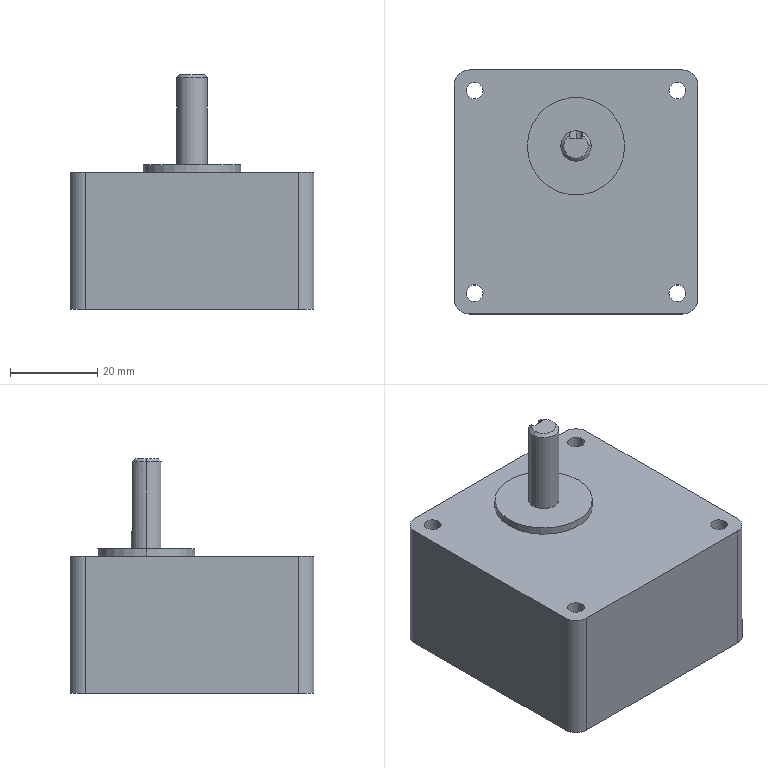Part | SolidWorks | features SplitBody 1 | 1 solid | 32 faces | box 56 x 56 x 53.9 mm | volume 98386 mm3 | cylinder 18 | plane 11 | cone 3 | commonest cylinder face diameters 3.85 x8 7 x6 2.8 x2 22.4 x2
STEP:
#1=CARTESIAN_POINT('',(-31.203,204.359,-234.916));
#2=VERTEX_POINT('',#1);
#3=CARTESIAN_POINT('',(-32.603,206.784,-234.916));
#4=VERTEX_POINT('',#3);
#5=CARTESIAN_POINT('',(-34.003,204.359,-234.916));
#6=DIRECTION('',(0.,0.,1.));
#7=DIRECTION('',(1.,0.,0.));
#8=AXIS2_PLACEMENT_3D('',#5,#6,#7);
#9=CIRCLE('',#8,2.8);
#10=EDGE_CURVE('',#2,#4,#9,.T.);
#11=ORIENTED_EDGE('',*,*,#10,.F.);
#12=CARTESIAN_POINT('',(-30.503,204.359,-235.616));
#13=VERTEX_POINT('',#12);
#14=CARTESIAN_POINT('',(-31.203,204.359,-234.916));
#15=DIRECTION('',(0.7071,0.,-0.7071));
#16=VECTOR('',#15,1000.);
#17=LINE('',#14,#16);
#18=EDGE_CURVE('',#2,#13,#17,.T.);
#19=ORIENTED_EDGE('',*,*,#18,.T.);
#20=CARTESIAN_POINT('',(-32.603,207.567,-235.616));
#21=VERTEX_POINT('',#20);
#22=CARTESIAN_POINT('',(-34.003,204.359,-235.616));
#23=DIRECTION('',(0.,0.,-1.));
#24=DIRECTION('',(1.,0.,0.));
#25=AXIS2_PLACEMENT_3D('',#22,#23,#24);
#26=CIRCLE('',#25,3.5);
#27=EDGE_CURVE('',#21,#13,#26,.T.);
#28=ORIENTED_EDGE('',*,*,#27,.F.);
#29=CARTESIAN_POINT('',(-32.603,206.784,-234.916));
#30=CARTESIAN_POINT('',(-32.603,207.049,-235.145));
#31=CARTESIAN_POINT('',(-32.603,207.309,-235.379));
#32=CARTESIAN_POINT('',(-32.603,207.567,-235.616));
#33=B_SPLINE_CURVE_WITH_KNOTS('',3,(#29,#30,#31,#32),.UNSPECIFIED.,.F.,.F.,(4,4),(0.002327,0.00337),.UNSPECIFIED.);
#34=EDGE_CURVE('',#4,#21,#33,.T.);
#35=ORIENTED_EDGE('',*,*,#34,.F.);
#36=EDGE_LOOP('',(#11,#19,#28,#35));
#37=FACE_OUTER_BOUND('',#36,.T.);
#38=CARTESIAN_POINT('',(-34.003,204.359,-234.916));
#39=DIRECTION('',(0.,0.,-1.));
#40=DIRECTION('',(-1.,0.,0.));
#41=AXIS2_PLACEMENT_3D('',#38,#39,#40);
#42=CONICAL_SURFACE('',#41,2.8,0.7854);
#43=ADVANCED_FACE('',(#37),#42,.T.);
#44=ORIENTED_EDGE('',*,*,#18,.F.);
#45=CARTESIAN_POINT('',(-36.803,204.359,-234.916));
#46=VERTEX_POINT('',#45);
#47=CARTESIAN_POINT('',(-34.003,204.359,-234.916));
#48=DIRECTION('',(0.,0.,1.));
#49=DIRECTION('',(1.,0.,0.));
#50=AXIS2_PLACEMENT_3D('',#47,#48,#49);
#51=CIRCLE('',#50,2.8);
#52=EDGE_CURVE('',#46,#2,#51,.T.);
#53=ORIENTED_EDGE('',*,*,#52,.F.);
#54=CARTESIAN_POINT('',(-37.503,204.359,-235.616));
#55=VERTEX_POINT('',#54);
#56=CARTESIAN_POINT('',(-36.803,204.359,-234.916));
#57=DIRECTION('',(-0.7071,0.,-0.7071));
#58=VECTOR('',#57,1000.);
#59=LINE('',#56,#58);
#60=EDGE_CURVE('',#46,#55,#59,.T.);
#61=ORIENTED_EDGE('',*,*,#60,.T.);
#62=CARTESIAN_POINT('',(-34.003,204.359,-235.616));
#63=DIRECTION('',(0.,0.,-1.));
#64=DIRECTION('',(1.,0.,0.));
#65=AXIS2_PLACEMENT_3D('',#62,#63,#64);
#66=CIRCLE('',#65,3.5);
#67=EDGE_CURVE('',#13,#55,#66,.T.);
#68=ORIENTED_EDGE('',*,*,#67,.F.);
#69=EDGE_LOOP('',(#44,#53,#61,#68));
#70=FACE_OUTER_BOUND('',#69,.T.);
#71=CARTESIAN_POINT('',(-34.003,204.359,-234.916));
#72=DIRECTION('',(0.,0.,-1.));
#73=DIRECTION('',(-1.,0.,0.));
#74=AXIS2_PLACEMENT_3D('',#71,#72,#73);
#75=CONICAL_SURFACE('',#74,2.8,0.7854);
#76=ADVANCED_FACE('',(#70),#75,.T.);
#77=ORIENTED_EDGE('',*,*,#27,.T.);
#78=CARTESIAN_POINT('',(-30.503,204.359,-255.566));
#79=VERTEX_POINT('',#78);
#80=CARTESIAN_POINT('',(-30.503,204.359,-234.916));
#81=DIRECTION('',(0.,0.,-1.));
#82=VECTOR('',#81,1000.);
#83=LINE('',#80,#82);
#84=EDGE_CURVE('',#13,#79,#83,.T.);
#85=ORIENTED_EDGE('',*,*,#84,.T.);
#86=CARTESIAN_POINT('',(-37.503,204.359,-255.566));
#87=VERTEX_POINT('',#86);
#88=CARTESIAN_POINT('',(-34.003,204.359,-255.566));
#89=DIRECTION('',(0.,0.,-1.));
#90=DIRECTION('',(1.,0.,0.));
#91=AXIS2_PLACEMENT_3D('',#88,#89,#90);
#92=CIRCLE('',#91,3.5);
#93=EDGE_CURVE('',#87,#79,#92,.T.);
#94=ORIENTED_EDGE('',*,*,#93,.F.);
#95=CARTESIAN_POINT('',(-37.503,204.359,-234.916));
#96=DIRECTION('',(0.,0.,-1.));
#97=VECTOR('',#96,1000.);
#98=LINE('',#95,#97);
#99=EDGE_CURVE('',#55,#87,#98,.T.);
#100=ORIENTED_EDGE('',*,*,#99,.F.);
#101=CARTESIAN_POINT('',(-35.403,207.567,-235.616));
#102=VERTEX_POINT('',#101);
#103=CARTESIAN_POINT('',(-34.003,204.359,-235.616));
#104=DIRECTION('',(0.,0.,-1.));
#105=DIRECTION('',(1.,0.,0.));
#106=AXIS2_PLACEMENT_3D('',#103,#104,#105);
#107=CIRCLE('',#106,3.5);
#108=EDGE_CURVE('',#55,#102,#107,.T.);
#109=ORIENTED_EDGE('',*,*,#108,.T.);
#110=CARTESIAN_POINT('',(-35.403,207.567,-251.016));
#111=VERTEX_POINT('',#110);
#112=CARTESIAN_POINT('',(-35.403,207.567,-234.916));
#113=DIRECTION('',(0.,0.,-1.));
#114=VECTOR('',#113,1000.);
#115=LINE('',#112,#114);
#116=EDGE_CURVE('',#102,#111,#115,.T.);
#117=ORIENTED_EDGE('',*,*,#116,.T.);
#118=CARTESIAN_POINT('',(-34.003,207.859,-252.416));
#119=VERTEX_POINT('',#118);
#120=CARTESIAN_POINT('',(-35.403,207.567,-251.016));
#121=CARTESIAN_POINT('',(-35.403,207.567,-251.109));
#122=CARTESIAN_POINT('',(-35.394,207.571,-251.201));
#123=CARTESIAN_POINT('',(-35.357,207.586,-251.381));
#124=CARTESIAN_POINT('',(-35.33,207.598,-251.47));
#125=CARTESIAN_POINT('',(-35.224,207.64,-251.724));
#126=CARTESIAN_POINT('',(-35.121,207.678,-251.877));
#127=CARTESIAN_POINT('',(-34.866,207.754,-252.133));
#128=CARTESIAN_POINT('',(-34.711,207.791,-252.237));
#129=CARTESIAN_POINT('',(-34.375,207.843,-252.377));
#130=CARTESIAN_POINT('',(-34.19,207.859,-252.416));
#131=CARTESIAN_POINT('',(-34.003,207.859,-252.416));
#132=B_SPLINE_CURVE_WITH_KNOTS('',3,(#120,#121,#122,#123,#124,#125,#126,#127,#128,#129,#130,#131),.UNSPECIFIED.,.F.,.F.,(4,2,2,2,2,4),(0.,0.0002763,0.0005526,0.001105,0.001658,0.00221),.UNSPECIFIED.);
#133=EDGE_CURVE('',#111,#119,#132,.T.);
#134=ORIENTED_EDGE('',*,*,#133,.T.);
#135=CARTESIAN_POINT('',(-32.603,207.567,-251.016));
#136=VERTEX_POINT('',#135);
#137=CARTESIAN_POINT('',(-34.003,207.859,-252.416));
#138=CARTESIAN_POINT('',(-33.909,207.859,-252.416));
#139=CARTESIAN_POINT('',(-33.818,207.855,-252.406));
#140=CARTESIAN_POINT('',(-33.637,207.841,-252.37));
#141=CARTESIAN_POINT('',(-33.548,207.83,-252.343));
#142=CARTESIAN_POINT('',(-33.294,207.791,-252.237));
#143=CARTESIAN_POINT('',(-33.14,207.754,-252.133));
#144=CARTESIAN_POINT('',(-32.885,207.678,-251.878));
#145=CARTESIAN_POINT('',(-32.781,207.64,-251.723));
#146=CARTESIAN_POINT('',(-32.641,207.584,-251.388));
#147=CARTESIAN_POINT('',(-32.603,207.567,-251.203));
#148=CARTESIAN_POINT('',(-32.603,207.567,-251.016));
#149=B_SPLINE_CURVE_WITH_KNOTS('',3,(#137,#138,#139,#140,#141,#142,#143,#144,#145,#146,#147,#148),.UNSPECIFIED.,.F.,.F.,(4,2,2,2,2,4),(0.,0.0002763,0.0005527,0.001105,0.001658,0.002211),.UNSPECIFIED.);
#150=EDGE_CURVE('',#119,#136,#149,.T.);
#151=ORIENTED_EDGE('',*,*,#150,.T.);
#152=CARTESIAN_POINT('',(-32.603,207.567,-234.916));
#153=DIRECTION('',(0.,0.,1.));
#154=VECTOR('',#153,1000.);
#155=LINE('',#152,#154);
#156=EDGE_CURVE('',#136,#21,#155,.T.);
#157=ORIENTED_EDGE('',*,*,#156,.T.);
#158=EDGE_LOOP('',(#77,#85,#94,#100,#109,#117,#134,#151,#157));
#159=FACE_OUTER_BOUND('',#158,.T.);
#160=CARTESIAN_POINT('',(-34.003,204.359,-234.916));
#161=DIRECTION('',(0.,0.,-1.));
#162=DIRECTION('',(-1.,0.,0.));
#163=AXIS2_PLACEMENT_3D('',#160,#161,#162);
#164=CYLINDRICAL_SURFACE('',#163,3.5);
#165=ADVANCED_FACE('',(#159),#164,.T.);
#166=CARTESIAN_POINT('',(-22.803,204.359,-255.566));
#167=VERTEX_POINT('',#166);
#168=CARTESIAN_POINT('',(-45.203,204.359,-255.566));
#169=VERTEX_POINT('',#168);
#170=CARTESIAN_POINT('',(-34.003,204.359,-255.566));
#171=DIRECTION('',(0.,0.,1.));
#172=DIRECTION('',(1.,0.,0.));
#173=AXIS2_PLACEMENT_3D('',#170,#171,#172);
#174=CIRCLE('',#173,11.2);
#175=EDGE_CURVE('',#167,#169,#174,.T.);
#176=ORIENTED_EDGE('',*,*,#175,.F.);
#177=CARTESIAN_POINT('',(-22.803,204.359,-257.316));
#178=VERTEX_POINT('',#177);
#179=CARTESIAN_POINT('',(-22.803,204.359,-255.566));
#180=DIRECTION('',(0.,0.,-1.));
#181=VECTOR('',#180,1000.);
#182=LINE('',#179,#181);
#183=EDGE_CURVE('',#167,#178,#182,.T.);
#184=ORIENTED_EDGE('',*,*,#183,.T.);
#185=CARTESIAN_POINT('',(-45.203,204.359,-257.316));
#186=VERTEX_POINT('',#185);
#187=CARTESIAN_POINT('',(-34.003,204.359,-257.316));
#188=DIRECTION('',(0.,0.,1.));
#189=DIRECTION('',(1.,0.,0.));
#190=AXIS2_PLACEMENT_3D('',#187,#188,#189);
#191=CIRCLE('',#190,11.2);
#192=EDGE_CURVE('',#178,#186,#191,.T.);
#193=ORIENTED_EDGE('',*,*,#192,.T.);
#194=CARTESIAN_POINT('',(-45.203,204.359,-255.566));
#195=DIRECTION('',(0.,0.,-1.));
#196=VECTOR('',#195,1000.);
#197=LINE('',#194,#196);
#198=EDGE_CURVE('',#169,#186,#197,.T.);
#199=ORIENTED_EDGE('',*,*,#198,.F.);
#200=EDGE_LOOP('',(#176,#184,#193,#199));
#201=FACE_OUTER_BOUND('',#200,.T.);
#202=CARTESIAN_POINT('',(-34.003,204.359,-255.566));
#203=DIRECTION('',(0.,0.,-1.));
#204=DIRECTION('',(-1.,0.,0.));
#205=AXIS2_PLACEMENT_3D('',#202,#203,#204);
#206=CYLINDRICAL_SURFACE('',#205,11.2);
#207=ADVANCED_FACE('',(#201),#206,.T.);
#208=CARTESIAN_POINT('',(-12.664,217.123,-257.316));
#209=VERTEX_POINT('',#208);
#210=CARTESIAN_POINT('',(-8.814,217.123,-257.316));
#211=VERTEX_POINT('',#210);
#212=CARTESIAN_POINT('',(-10.739,217.123,-257.316));
#213=DIRECTION('',(0.,0.,1.));
#214=DIRECTION('',(1.,0.,0.));
#215=AXIS2_PLACEMENT_3D('',#212,#213,#214);
#216=CIRCLE('',#215,1.925);
#217=EDGE_CURVE('',#209,#211,#216,.T.);
#218=ORIENTED_EDGE('',*,*,#217,.T.);
#219=CARTESIAN_POINT('',(-8.814,217.123,-288.816));
#220=VERTEX_POINT('',#219);
#221=CARTESIAN_POINT('',(-8.814,217.123,-257.316));
#222=DIRECTION('',(0.,0.,-1.));
#223=VECTOR('',#222,1000.);
#224=LINE('',#221,#223);
#225=EDGE_CURVE('',#211,#220,#224,.T.);
#226=ORIENTED_EDGE('',*,*,#225,.T.);
#227=CARTESIAN_POINT('',(-12.664,217.123,-288.816));
#228=VERTEX_POINT('',#227);
#229=CARTESIAN_POINT('',(-10.739,217.123,-288.816));
#230=DIRECTION('',(0.,0.,1.));
#231=DIRECTION('',(1.,0.,0.));
#232=AXIS2_PLACEMENT_3D('',#229,#230,#231);
#233=CIRCLE('',#232,1.925);
#234=EDGE_CURVE('',#228,#220,#233,.T.);
#235=ORIENTED_EDGE('',*,*,#234,.F.);
#236=CARTESIAN_POINT('',(-12.664,217.123,-257.316));
#237=DIRECTION('',(0.,0.,-1.));
#238=VECTOR('',#237,1000.);
#239=LINE('',#236,#238);
#240=EDGE_CURVE('',#209,#228,#239,.T.);
#241=ORIENTED_EDGE('',*,*,#240,.F.);
#242=EDGE_LOOP('',(#218,#226,#235,#241));
#243=FACE_OUTER_BOUND('',#242,.T.);
#244=CARTESIAN_POINT('',(-10.739,217.123,-257.316));
#245=DIRECTION('',(0.,0.,-1.));
#246=DIRECTION('',(-1.,0.,0.));
#247=AXIS2_PLACEMENT_3D('',#244,#245,#246);
#248=CYLINDRICAL_SURFACE('',#247,1.925);
#249=ADVANCED_FACE('',(#243),#248,.F.);
#250=CARTESIAN_POINT('',(-12.664,170.595,-257.316));
#251=VERTEX_POINT('',#250);
#252=CARTESIAN_POINT('',(-8.814,170.595,-257.316));
#253=VERTEX_POINT('',#252);
#254=CARTESIAN_POINT('',(-10.739,170.595,-257.316));
#255=DIRECTION('',(0.,0.,1.));
#256=DIRECTION('',(1.,0.,0.));
#257=AXIS2_PLACEMENT_3D('',#254,#255,#256);
#258=CIRCLE('',#257,1.925);
#259=EDGE_CURVE('',#251,#253,#258,.T.);
#260=ORIENTED_EDGE('',*,*,#259,.T.);
#261=CARTESIAN_POINT('',(-8.814,170.595,-288.816));
#262=VERTEX_POINT('',#261);
#263=CARTESIAN_POINT('',(-8.814,170.595,-257.316));
#264=DIRECTION('',(0.,0.,-1.));
#265=VECTOR('',#264,1000.);
#266=LINE('',#263,#265);
#267=EDGE_CURVE('',#253,#262,#266,.T.);
#268=ORIENTED_EDGE('',*,*,#267,.T.);
#269=CARTESIAN_POINT('',(-12.664,170.595,-288.816));
#270=VERTEX_POINT('',#269);
#271=CARTESIAN_POINT('',(-10.739,170.595,-288.816));
#272=DIRECTION('',(0.,0.,1.));
#273=DIRECTION('',(1.,0.,0.));
#274=AXIS2_PLACEMENT_3D('',#271,#272,#273);
#275=CIRCLE('',#274,1.925);
#276=EDGE_CURVE('',#270,#262,#275,.T.);
#277=ORIENTED_EDGE('',*,*,#276,.F.);
#278=CARTESIAN_POINT('',(-12.664,170.595,-257.316));
#279=DIRECTION('',(0.,0.,-1.));
#280=VECTOR('',#279,1000.);
#281=LINE('',#278,#280);
#282=EDGE_CURVE('',#251,#270,#281,.T.);
#283=ORIENTED_EDGE('',*,*,#282,.F.);
#284=EDGE_LOOP('',(#260,#268,#277,#283));
#285=FACE_OUTER_BOUND('',#284,.T.);
#286=CARTESIAN_POINT('',(-10.739,170.595,-257.316));
#287=DIRECTION('',(0.,0.,-1.));
#288=DIRECTION('',(-1.,0.,0.));
#289=AXIS2_PLACEMENT_3D('',#286,#287,#288);
#290=CYLINDRICAL_SURFACE('',#289,1.925);
#291=ADVANCED_FACE('',(#285),#290,.F.);
#292=CARTESIAN_POINT('',(-59.192,170.595,-257.316));
#293=VERTEX_POINT('',#292);
#294=CARTESIAN_POINT('',(-55.342,170.595,-257.316));
#295=VERTEX_POINT('',#294);
#296=CARTESIAN_POINT('',(-57.267,170.595,-257.316));
#297=DIRECTION('',(0.,0.,1.));
#298=DIRECTION('',(1.,0.,0.));
#299=AXIS2_PLACEMENT_3D('',#296,#297,#298);
#300=CIRCLE('',#299,1.925);
#301=EDGE_CURVE('',#293,#295,#300,.T.);
#302=ORIENTED_EDGE('',*,*,#301,.T.);
#303=CARTESIAN_POINT('',(-55.342,170.595,-288.816));
#304=VERTEX_POINT('',#303);
#305=CARTESIAN_POINT('',(-55.342,170.595,-257.316));
#306=DIRECTION('',(0.,0.,-1.));
#307=VECTOR('',#306,1000.);
#308=LINE('',#305,#307);
#309=EDGE_CURVE('',#295,#304,#308,.T.);
#310=ORIENTED_EDGE('',*,*,#309,.T.);
#311=CARTESIAN_POINT('',(-59.192,170.595,-288.816));
#312=VERTEX_POINT('',#311);
#313=CARTESIAN_POINT('',(-57.267,170.595,-288.816));
#314=DIRECTION('',(0.,0.,1.));
#315=DIRECTION('',(1.,0.,0.));
#316=AXIS2_PLACEMENT_3D('',#313,#314,#315);
#317=CIRCLE('',#316,1.925);
#318=EDGE_CURVE('',#312,#304,#317,.T.);
#319=ORIENTED_EDGE('',*,*,#318,.F.);
#320=CARTESIAN_POINT('',(-59.192,170.595,-257.316));
#321=DIRECTION('',(0.,0.,-1.));
#322=VECTOR('',#321,1000.);
#323=LINE('',#320,#322);
#324=EDGE_CURVE('',#293,#312,#323,.T.);
#325=ORIENTED_EDGE('',*,*,#324,.F.);
#326=EDGE_LOOP('',(#302,#310,#319,#325));
#327=FACE_OUTER_BOUND('',#326,.T.);
#328=CARTESIAN_POINT('',(-57.267,170.595,-257.316));
#329=DIRECTION('',(0.,0.,-1.));
#330=DIRECTION('',(-1.,0.,0.));
#331=AXIS2_PLACEMENT_3D('',#328,#329,#330);
#332=CYLINDRICAL_SURFACE('',#331,1.925);
#333=ADVANCED_FACE('',(#327),#332,.F.);
#334=CARTESIAN_POINT('',(-59.192,217.123,-257.316));
#335=VERTEX_POINT('',#334);
#336=CARTESIAN_POINT('',(-55.342,217.123,-257.316));
#337=VERTEX_POINT('',#336);
#338=CARTESIAN_POINT('',(-57.267,217.123,-257.316));
#339=DIRECTION('',(0.,0.,1.));
#340=DIRECTION('',(1.,0.,0.));
#341=AXIS2_PLACEMENT_3D('',#338,#339,#340);
#342=CIRCLE('',#341,1.925);
#343=EDGE_CURVE('',#335,#337,#342,.T.);
#344=ORIENTED_EDGE('',*,*,#343,.T.);
#345=CARTESIAN_POINT('',(-55.342,217.123,-288.816));
#346=VERTEX_POINT('',#345);
#347=CARTESIAN_POINT('',(-55.342,217.123,-257.316));
#348=DIRECTION('',(0.,0.,-1.));
#349=VECTOR('',#348,1000.);
#350=LINE('',#347,#349);
#351=EDGE_CURVE('',#337,#346,#350,.T.);
#352=ORIENTED_EDGE('',*,*,#351,.T.);
#353=CARTESIAN_POINT('',(-59.192,217.123,-288.816));
#354=VERTEX_POINT('',#353);
#355=CARTESIAN_POINT('',(-57.267,217.123,-288.816));
#356=DIRECTION('',(0.,0.,1.));
#357=DIRECTION('',(1.,0.,0.));
#358=AXIS2_PLACEMENT_3D('',#355,#356,#357);
#359=CIRCLE('',#358,1.925);
#360=EDGE_CURVE('',#354,#346,#359,.T.);
#361=ORIENTED_EDGE('',*,*,#360,.F.);
#362=CARTESIAN_POINT('',(-59.192,217.123,-257.316));
#363=DIRECTION('',(0.,0.,-1.));
#364=VECTOR('',#363,1000.);
#365=LINE('',#362,#364);
#366=EDGE_CURVE('',#335,#354,#365,.T.);
#367=ORIENTED_EDGE('',*,*,#366,.F.);
#368=EDGE_LOOP('',(#344,#352,#361,#367));
#369=FACE_OUTER_BOUND('',#368,.T.);
#370=CARTESIAN_POINT('',(-57.267,217.123,-257.316));
#371=DIRECTION('',(0.,0.,-1.));
#372=DIRECTION('',(-1.,0.,0.));
#373=AXIS2_PLACEMENT_3D('',#370,#371,#372);
#374=CYLINDRICAL_SURFACE('',#373,1.925);
#375=ADVANCED_FACE('',(#369),#374,.F.);
#376=CARTESIAN_POINT('',(-34.003,204.359,-255.566));
#377=DIRECTION('',(0.,0.,1.));
#378=DIRECTION('',(1.,0.,0.));
#379=AXIS2_PLACEMENT_3D('',#376,#377,#378);
#380=CIRCLE('',#379,11.2);
#381=EDGE_CURVE('',#169,#167,#380,.T.);
#382=ORIENTED_EDGE('',*,*,#381,.T.);
#383=ORIENTED_EDGE('',*,*,#175,.T.);
#384=EDGE_LOOP('',(#382,#383));
#385=FACE_OUTER_BOUND('',#384,.T.);
#386=ORIENTED_EDGE('',*,*,#93,.T.);
#387=CARTESIAN_POINT('',(-34.003,204.359,-255.566));
#388=DIRECTION('',(0.,0.,-1.));
#389=DIRECTION('',(1.,0.,0.));
#390=AXIS2_PLACEMENT_3D('',#387,#388,#389);
#391=CIRCLE('',#390,3.5);
#392=EDGE_CURVE('',#79,#87,#391,.T.);
#393=ORIENTED_EDGE('',*,*,#392,.T.);
#394=EDGE_LOOP('',(#386,#393));
#395=FACE_BOUND('',#394,.T.);
#396=CARTESIAN_POINT('',(-34.003,204.359,-255.566));
#397=DIRECTION('',(0.,0.,1.));
#398=DIRECTION('',(1.,0.,0.));
#399=AXIS2_PLACEMENT_3D('',#396,#397,#398);
#400=PLANE('',#399);
#401=ADVANCED_FACE('',(#385,#395),#400,.T.);
#402=ORIENTED_EDGE('',*,*,#217,.F.);
#403=CARTESIAN_POINT('',(-10.739,217.123,-257.316));
#404=DIRECTION('',(0.,0.,1.));
#405=DIRECTION('',(1.,0.,0.));
#406=AXIS2_PLACEMENT_3D('',#403,#404,#405);
#407=CIRCLE('',#406,1.925);
#408=EDGE_CURVE('',#211,#209,#407,.T.);
#409=ORIENTED_EDGE('',*,*,#408,.F.);
#410=EDGE_LOOP('',(#402,#409));
#411=FACE_BOUND('',#410,.T.);
#412=ORIENTED_EDGE('',*,*,#301,.F.);
#413=CARTESIAN_POINT('',(-57.267,170.595,-257.316));
#414=DIRECTION('',(0.,0.,1.));
#415=DIRECTION('',(1.,0.,0.));
#416=AXIS2_PLACEMENT_3D('',#413,#414,#415);
#417=CIRCLE('',#416,1.925);
#418=EDGE_CURVE('',#295,#293,#417,.T.);
#419=ORIENTED_EDGE('',*,*,#418,.F.);
#420=EDGE_LOOP('',(#412,#419));
#421=FACE_BOUND('',#420,.T.);
#422=CARTESIAN_POINT('',(-62.003,169.359,-257.316));
#423=VERTEX_POINT('',#422);
#424=CARTESIAN_POINT('',(-58.503,165.859,-257.316));
#425=VERTEX_POINT('',#424);
#426=CARTESIAN_POINT('',(-58.503,169.359,-257.316));
#427=DIRECTION('',(0.,0.,1.));
#428=DIRECTION('',(1.,0.,0.));
#429=AXIS2_PLACEMENT_3D('',#426,#427,#428);
#430=CIRCLE('',#429,3.5);
#431=EDGE_CURVE('',#423,#425,#430,.T.);
#432=ORIENTED_EDGE('',*,*,#431,.T.);
#433=CARTESIAN_POINT('',(-9.503,165.859,-257.316));
#434=VERTEX_POINT('',#433);
#435=CARTESIAN_POINT('',(-58.503,165.859,-257.316));
#436=DIRECTION('',(1.,0.,0.));
#437=VECTOR('',#436,1000.);
#438=LINE('',#435,#437);
#439=EDGE_CURVE('',#425,#434,#438,.T.);
#440=ORIENTED_EDGE('',*,*,#439,.T.);
#441=CARTESIAN_POINT('',(-6.003,169.359,-257.316));
#442=VERTEX_POINT('',#441);
#443=CARTESIAN_POINT('',(-9.503,169.359,-257.316));
#444=DIRECTION('',(0.,0.,1.));
#445=DIRECTION('',(1.,0.,0.));
#446=AXIS2_PLACEMENT_3D('',#443,#444,#445);
#447=CIRCLE('',#446,3.5);
#448=EDGE_CURVE('',#434,#442,#447,.T.);
#449=ORIENTED_EDGE('',*,*,#448,.T.);
#450=CARTESIAN_POINT('',(-6.003,218.359,-257.316));
#451=VERTEX_POINT('',#450);
#452=CARTESIAN_POINT('',(-6.003,169.359,-257.316));
#453=DIRECTION('',(0.,1.,0.));
#454=VECTOR('',#453,1000.);
#455=LINE('',#452,#454);
#456=EDGE_CURVE('',#442,#451,#455,.T.);
#457=ORIENTED_EDGE('',*,*,#456,.T.);
#458=CARTESIAN_POINT('',(-9.503,221.859,-257.316));
#459=VERTEX_POINT('',#458);
#460=CARTESIAN_POINT('',(-9.503,218.359,-257.316));
#461=DIRECTION('',(0.,0.,1.));
#462=DIRECTION('',(1.,0.,0.));
#463=AXIS2_PLACEMENT_3D('',#460,#461,#462);
#464=CIRCLE('',#463,3.5);
#465=EDGE_CURVE('',#451,#459,#464,.T.);
#466=ORIENTED_EDGE('',*,*,#465,.T.);
#467=CARTESIAN_POINT('',(-58.503,221.859,-257.316));
#468=VERTEX_POINT('',#467);
#469=CARTESIAN_POINT('',(-9.503,221.859,-257.316));
#470=DIRECTION('',(-1.,0.,0.));
#471=VECTOR('',#470,1000.);
#472=LINE('',#469,#471);
#473=EDGE_CURVE('',#459,#468,#472,.T.);
#474=ORIENTED_EDGE('',*,*,#473,.T.);
#475=CARTESIAN_POINT('',(-62.003,218.359,-257.316));
#476=VERTEX_POINT('',#475);
#477=CARTESIAN_POINT('',(-58.503,218.359,-257.316));
#478=DIRECTION('',(0.,0.,1.));
#479=DIRECTION('',(1.,0.,0.));
#480=AXIS2_PLACEMENT_3D('',#477,#478,#479);
#481=CIRCLE('',#480,3.5);
#482=EDGE_CURVE('',#468,#476,#481,.T.);
#483=ORIENTED_EDGE('',*,*,#482,.T.);
#484=CARTESIAN_POINT('',(-62.003,218.359,-257.316));
#485=DIRECTION('',(0.,-1.,0.));
#486=VECTOR('',#485,1000.);
#487=LINE('',#484,#486);
#488=EDGE_CURVE('',#476,#423,#487,.T.);
#489=ORIENTED_EDGE('',*,*,#488,.T.);
#490=EDGE_LOOP('',(#432,#440,#449,#457,#466,#474,#483,#489));
#491=FACE_OUTER_BOUND('',#490,.T.);
#492=ORIENTED_EDGE('',*,*,#343,.F.);
#493=CARTESIAN_POINT('',(-57.267,217.123,-257.316));
#494=DIRECTION('',(0.,0.,1.));
#495=DIRECTION('',(1.,0.,0.));
#496=AXIS2_PLACEMENT_3D('',#493,#494,#495);
#497=CIRCLE('',#496,1.925);
#498=EDGE_CURVE('',#337,#335,#497,.T.);
#499=ORIENTED_EDGE('',*,*,#498,.F.);
#500=EDGE_LOOP('',(#492,#499));
#501=FACE_BOUND('',#500,.T.);
#502=ORIENTED_EDGE('',*,*,#259,.F.);
#503=CARTESIAN_POINT('',(-10.739,170.595,-257.316));
#504=DIRECTION('',(0.,0.,1.));
#505=DIRECTION('',(1.,0.,0.));
#506=AXIS2_PLACEMENT_3D('',#503,#504,#505);
#507=CIRCLE('',#506,1.925);
#508=EDGE_CURVE('',#253,#251,#507,.T.);
#509=ORIENTED_EDGE('',*,*,#508,.F.);
#510=EDGE_LOOP('',(#502,#509));
#511=FACE_BOUND('',#510,.T.);
#512=CARTESIAN_POINT('',(-34.003,204.359,-257.316));
#513=DIRECTION('',(0.,0.,1.));
#514=DIRECTION('',(1.,0.,0.));
#515=AXIS2_PLACEMENT_3D('',#512,#513,#514);
#516=CIRCLE('',#515,11.2);
#517=EDGE_CURVE('',#186,#178,#516,.T.);
#518=ORIENTED_EDGE('',*,*,#517,.F.);
#519=ORIENTED_EDGE('',*,*,#192,.F.);
#520=EDGE_LOOP('',(#518,#519));
#521=FACE_BOUND('',#520,.T.);
#522=CARTESIAN_POINT('',(-58.503,169.359,-257.316));
#523=DIRECTION('',(0.,0.,1.));
#524=DIRECTION('',(1.,0.,0.));
#525=AXIS2_PLACEMENT_3D('',#522,#523,#524);
#526=PLANE('',#525);
#527=ADVANCED_FACE('',(#411,#421,#491,#501,#511,#521),#526,.T.);
#528=ORIENTED_EDGE('',*,*,#276,.T.);
#529=CARTESIAN_POINT('',(-10.739,170.595,-288.816));
#530=DIRECTION('',(0.,0.,1.));
#531=DIRECTION('',(1.,0.,0.));
#532=AXIS2_PLACEMENT_3D('',#529,#530,#531);
#533=CIRCLE('',#532,1.925);
#534=EDGE_CURVE('',#262,#270,#533,.T.);
#535=ORIENTED_EDGE('',*,*,#534,.T.);
#536=EDGE_LOOP('',(#528,#535));
#537=FACE_BOUND('',#536,.T.);
#538=ORIENTED_EDGE('',*,*,#360,.T.);
#539=CARTESIAN_POINT('',(-57.267,217.123,-288.816));
#540=DIRECTION('',(0.,0.,1.));
#541=DIRECTION('',(1.,0.,0.));
#542=AXIS2_PLACEMENT_3D('',#539,#540,#541);
#543=CIRCLE('',#542,1.925);
#544=EDGE_CURVE('',#346,#354,#543,.T.);
#545=ORIENTED_EDGE('',*,*,#544,.T.);
#546=EDGE_LOOP('',(#538,#545));
#547=FACE_BOUND('',#546,.T.);
#548=CARTESIAN_POINT('',(-62.003,169.359,-288.816));
#549=VERTEX_POINT('',#548);
#550=CARTESIAN_POINT('',(-58.503,165.859,-288.816));
#551=VERTEX_POINT('',#550);
#552=CARTESIAN_POINT('',(-58.503,169.359,-288.816));
#553=DIRECTION('',(0.,0.,1.));
#554=DIRECTION('',(1.,0.,0.));
#555=AXIS2_PLACEMENT_3D('',#552,#553,#554);
#556=CIRCLE('',#555,3.5);
#557=EDGE_CURVE('',#549,#551,#556,.T.);
#558=ORIENTED_EDGE('',*,*,#557,.F.);
#559=CARTESIAN_POINT('',(-62.003,218.359,-288.816));
#560=VERTEX_POINT('',#559);
#561=CARTESIAN_POINT('',(-62.003,218.359,-288.816));
#562=DIRECTION('',(0.,-1.,0.));
#563=VECTOR('',#562,1000.);
#564=LINE('',#561,#563);
#565=EDGE_CURVE('',#560,#549,#564,.T.);
#566=ORIENTED_EDGE('',*,*,#565,.F.);
#567=CARTESIAN_POINT('',(-58.503,221.859,-288.816));
#568=VERTEX_POINT('',#567);
#569=CARTESIAN_POINT('',(-58.503,218.359,-288.816));
#570=DIRECTION('',(0.,0.,1.));
#571=DIRECTION('',(1.,0.,0.));
#572=AXIS2_PLACEMENT_3D('',#569,#570,#571);
#573=CIRCLE('',#572,3.5);
#574=EDGE_CURVE('',#568,#560,#573,.T.);
#575=ORIENTED_EDGE('',*,*,#574,.F.);
#576=CARTESIAN_POINT('',(-9.503,221.859,-288.816));
#577=VERTEX_POINT('',#576);
#578=CARTESIAN_POINT('',(-9.503,221.859,-288.816));
#579=DIRECTION('',(-1.,0.,0.));
#580=VECTOR('',#579,1000.);
#581=LINE('',#578,#580);
#582=EDGE_CURVE('',#577,#568,#581,.T.);
#583=ORIENTED_EDGE('',*,*,#582,.F.);
#584=CARTESIAN_POINT('',(-6.003,218.359,-288.816));
#585=VERTEX_POINT('',#584);
#586=CARTESIAN_POINT('',(-9.503,218.359,-288.816));
#587=DIRECTION('',(0.,0.,1.));
#588=DIRECTION('',(1.,0.,0.));
#589=AXIS2_PLACEMENT_3D('',#586,#587,#588);
#590=CIRCLE('',#589,3.5);
#591=EDGE_CURVE('',#585,#577,#590,.T.);
#592=ORIENTED_EDGE('',*,*,#591,.F.);
#593=CARTESIAN_POINT('',(-6.003,169.359,-288.816));
#594=VERTEX_POINT('',#593);
#595=CARTESIAN_POINT('',(-6.003,169.359,-288.816));
#596=DIRECTION('',(0.,1.,0.));
#597=VECTOR('',#596,1000.);
#598=LINE('',#595,#597);
#599=EDGE_CURVE('',#594,#585,#598,.T.);
#600=ORIENTED_EDGE('',*,*,#599,.F.);
#601=CARTESIAN_POINT('',(-9.503,165.859,-288.816));
#602=VERTEX_POINT('',#601);
#603=CARTESIAN_POINT('',(-9.503,169.359,-288.816));
#604=DIRECTION('',(0.,0.,1.));
#605=DIRECTION('',(1.,0.,0.));
#606=AXIS2_PLACEMENT_3D('',#603,#604,#605);
#607=CIRCLE('',#606,3.5);
#608=EDGE_CURVE('',#602,#594,#607,.T.);
#609=ORIENTED_EDGE('',*,*,#608,.F.);
#610=CARTESIAN_POINT('',(-58.503,165.859,-288.816));
#611=DIRECTION('',(1.,0.,0.));
#612=VECTOR('',#611,1000.);
#613=LINE('',#610,#612);
#614=EDGE_CURVE('',#551,#602,#613,.T.);
#615=ORIENTED_EDGE('',*,*,#614,.F.);
#616=EDGE_LOOP('',(#558,#566,#575,#583,#592,#600,#609,#615));
#617=FACE_OUTER_BOUND('',#616,.T.);
#618=ORIENTED_EDGE('',*,*,#318,.T.);
#619=CARTESIAN_POINT('',(-57.267,170.595,-288.816));
#620=DIRECTION('',(0.,0.,1.));
#621=DIRECTION('',(1.,0.,0.));
#622=AXIS2_PLACEMENT_3D('',#619,#620,#621);
#623=CIRCLE('',#622,1.925);
#624=EDGE_CURVE('',#304,#312,#623,.T.);
#625=ORIENTED_EDGE('',*,*,#624,.T.);
#626=EDGE_LOOP('',(#618,#625));
#627=FACE_BOUND('',#626,.T.);
#628=ORIENTED_EDGE('',*,*,#234,.T.);
#629=CARTESIAN_POINT('',(-10.739,217.123,-288.816));
#630=DIRECTION('',(0.,0.,1.));
#631=DIRECTION('',(1.,0.,0.));
#632=AXIS2_PLACEMENT_3D('',#629,#630,#631);
#633=CIRCLE('',#632,1.925);
#634=EDGE_CURVE('',#220,#228,#633,.T.);
#635=ORIENTED_EDGE('',*,*,#634,.T.);
#636=EDGE_LOOP('',(#628,#635));
#637=FACE_BOUND('',#636,.T.);
#638=CARTESIAN_POINT('',(-58.503,169.359,-288.816));
#639=DIRECTION('',(0.,0.,1.));
#640=DIRECTION('',(1.,0.,0.));
#641=AXIS2_PLACEMENT_3D('',#638,#639,#640);
#642=PLANE('',#641);
#643=ADVANCED_FACE('',(#537,#547,#617,#627,#637),#642,.F.);
#644=ORIENTED_EDGE('',*,*,#557,.T.);
#645=CARTESIAN_POINT('',(-58.503,165.859,-257.316));
#646=DIRECTION('',(0.,0.,-1.));
#647=VECTOR('',#646,1000.);
#648=LINE('',#645,#647);
#649=EDGE_CURVE('',#425,#551,#648,.T.);
#650=ORIENTED_EDGE('',*,*,#649,.F.);
#651=ORIENTED_EDGE('',*,*,#431,.F.);
#652=CARTESIAN_POINT('',(-62.003,169.359,-257.316));
#653=DIRECTION('',(0.,0.,-1.));
#654=VECTOR('',#653,1000.);
#655=LINE('',#652,#654);
#656=EDGE_CURVE('',#423,#549,#655,.T.);
#657=ORIENTED_EDGE('',*,*,#656,.T.);
#658=EDGE_LOOP('',(#644,#650,#651,#657));
#659=FACE_OUTER_BOUND('',#658,.T.);
#660=CARTESIAN_POINT('',(-58.503,169.359,-257.316));
#661=DIRECTION('',(0.,0.,-1.));
#662=DIRECTION('',(-1.,0.,0.));
#663=AXIS2_PLACEMENT_3D('',#660,#661,#662);
#664=CYLINDRICAL_SURFACE('',#663,3.5);
#665=ADVANCED_FACE('',(#659),#664,.T.);
#666=ORIENTED_EDGE('',*,*,#614,.T.);
#667=CARTESIAN_POINT('',(-9.503,165.859,-257.316));
#668=DIRECTION('',(0.,0.,-1.));
#669=VECTOR('',#668,1000.);
#670=LINE('',#667,#669);
#671=EDGE_CURVE('',#434,#602,#670,.T.);
#672=ORIENTED_EDGE('',*,*,#671,.F.);
#673=ORIENTED_EDGE('',*,*,#439,.F.);
#674=ORIENTED_EDGE('',*,*,#649,.T.);
#675=EDGE_LOOP('',(#666,#672,#673,#674));
#676=FACE_OUTER_BOUND('',#675,.T.);
#677=CARTESIAN_POINT('',(-58.503,165.859,-257.316));
#678=DIRECTION('',(0.,1.,0.));
#679=DIRECTION('',(0.,0.,1.));
#680=AXIS2_PLACEMENT_3D('',#677,#678,#679);
#681=PLANE('',#680);
#682=ADVANCED_FACE('',(#676),#681,.F.);
#683=ORIENTED_EDGE('',*,*,#608,.T.);
#684=CARTESIAN_POINT('',(-6.003,169.359,-257.316));
#685=DIRECTION('',(0.,0.,-1.));
#686=VECTOR('',#685,1000.);
#687=LINE('',#684,#686);
#688=EDGE_CURVE('',#442,#594,#687,.T.);
#689=ORIENTED_EDGE('',*,*,#688,.F.);
#690=ORIENTED_EDGE('',*,*,#448,.F.);
#691=ORIENTED_EDGE('',*,*,#671,.T.);
#692=EDGE_LOOP('',(#683,#689,#690,#691));
#693=FACE_OUTER_BOUND('',#692,.T.);
#694=CARTESIAN_POINT('',(-9.503,169.359,-257.316));
#695=DIRECTION('',(0.,0.,-1.));
#696=DIRECTION('',(-1.,0.,0.));
#697=AXIS2_PLACEMENT_3D('',#694,#695,#696);
#698=CYLINDRICAL_SURFACE('',#697,3.5);
#699=ADVANCED_FACE('',(#693),#698,.T.);
#700=ORIENTED_EDGE('',*,*,#599,.T.);
#701=CARTESIAN_POINT('',(-6.003,218.359,-257.316));
#702=DIRECTION('',(0.,0.,-1.));
#703=VECTOR('',#702,1000.);
#704=LINE('',#701,#703);
#705=EDGE_CURVE('',#451,#585,#704,.T.);
#706=ORIENTED_EDGE('',*,*,#705,.F.);
#707=ORIENTED_EDGE('',*,*,#456,.F.);
#708=ORIENTED_EDGE('',*,*,#688,.T.);
#709=EDGE_LOOP('',(#700,#706,#707,#708));
#710=FACE_OUTER_BOUND('',#709,.T.);
#711=CARTESIAN_POINT('',(-6.003,169.359,-257.316));
#712=DIRECTION('',(-1.,0.,0.));
#713=DIRECTION('',(0.,-1.,0.));
#714=AXIS2_PLACEMENT_3D('',#711,#712,#713);
#715=PLANE('',#714);
#716=ADVANCED_FACE('',(#710),#715,.F.);
#717=ORIENTED_EDGE('',*,*,#591,.T.);
#718=CARTESIAN_POINT('',(-9.503,221.859,-257.316));
#719=DIRECTION('',(0.,0.,-1.));
#720=VECTOR('',#719,1000.);
#721=LINE('',#718,#720);
#722=EDGE_CURVE('',#459,#577,#721,.T.);
#723=ORIENTED_EDGE('',*,*,#722,.F.);
#724=ORIENTED_EDGE('',*,*,#465,.F.);
#725=ORIENTED_EDGE('',*,*,#705,.T.);
#726=EDGE_LOOP('',(#717,#723,#724,#725));
#727=FACE_OUTER_BOUND('',#726,.T.);
#728=CARTESIAN_POINT('',(-9.503,218.359,-257.316));
#729=DIRECTION('',(0.,0.,-1.));
#730=DIRECTION('',(-1.,0.,0.));
#731=AXIS2_PLACEMENT_3D('',#728,#729,#730);
#732=CYLINDRICAL_SURFACE('',#731,3.5);
#733=ADVANCED_FACE('',(#727),#732,.T.);
#734=ORIENTED_EDGE('',*,*,#582,.T.);
#735=CARTESIAN_POINT('',(-58.503,221.859,-257.316));
#736=DIRECTION('',(0.,0.,-1.));
#737=VECTOR('',#736,1000.);
#738=LINE('',#735,#737);
#739=EDGE_CURVE('',#468,#568,#738,.T.);
#740=ORIENTED_EDGE('',*,*,#739,.F.);
#741=ORIENTED_EDGE('',*,*,#473,.F.);
#742=ORIENTED_EDGE('',*,*,#722,.T.);
#743=EDGE_LOOP('',(#734,#740,#741,#742));
#744=FACE_OUTER_BOUND('',#743,.T.);
#745=CARTESIAN_POINT('',(-9.503,221.859,-257.316));
#746=DIRECTION('',(0.,-1.,0.));
#747=DIRECTION('',(0.,0.,-1.));
#748=AXIS2_PLACEMENT_3D('',#745,#746,#747);
#749=PLANE('',#748);
#750=ADVANCED_FACE('',(#744),#749,.F.);
#751=ORIENTED_EDGE('',*,*,#574,.T.);
#752=CARTESIAN_POINT('',(-62.003,218.359,-257.316));
#753=DIRECTION('',(0.,0.,-1.));
#754=VECTOR('',#753,1000.);
#755=LINE('',#752,#754);
#756=EDGE_CURVE('',#476,#560,#755,.T.);
#757=ORIENTED_EDGE('',*,*,#756,.F.);
#758=ORIENTED_EDGE('',*,*,#482,.F.);
#759=ORIENTED_EDGE('',*,*,#739,.T.);
#760=EDGE_LOOP('',(#751,#757,#758,#759));
#761=FACE_OUTER_BOUND('',#760,.T.);
#762=CARTESIAN_POINT('',(-58.503,218.359,-257.316));
#763=DIRECTION('',(0.,0.,-1.));
#764=DIRECTION('',(-1.,0.,0.));
#765=AXIS2_PLACEMENT_3D('',#762,#763,#764);
#766=CYLINDRICAL_SURFACE('',#765,3.5);
#767=ADVANCED_FACE('',(#761),#766,.T.);
#768=ORIENTED_EDGE('',*,*,#565,.T.);
#769=ORIENTED_EDGE('',*,*,#656,.F.);
#770=ORIENTED_EDGE('',*,*,#488,.F.);
#771=ORIENTED_EDGE('',*,*,#756,.T.);
#772=EDGE_LOOP('',(#768,#769,#770,#771));
#773=FACE_OUTER_BOUND('',#772,.T.);
#774=CARTESIAN_POINT('',(-62.003,218.359,-257.316));
#775=DIRECTION('',(1.,0.,0.));
#776=DIRECTION('',(0.,1.,0.));
#777=AXIS2_PLACEMENT_3D('',#774,#775,#776);
#778=PLANE('',#777);
#779=ADVANCED_FACE('',(#773),#778,.F.);
#780=ORIENTED_EDGE('',*,*,#351,.F.);
#781=ORIENTED_EDGE('',*,*,#498,.T.);
#782=ORIENTED_EDGE('',*,*,#366,.T.);
#783=ORIENTED_EDGE('',*,*,#544,.F.);
#784=EDGE_LOOP('',(#780,#781,#782,#783));
#785=FACE_OUTER_BOUND('',#784,.T.);
#786=CARTESIAN_POINT('',(-57.267,217.123,-257.316));
#787=DIRECTION('',(0.,0.,-1.));
#788=DIRECTION('',(-1.,0.,0.));
#789=AXIS2_PLACEMENT_3D('',#786,#787,#788);
#790=CYLINDRICAL_SURFACE('',#789,1.925);
#791=ADVANCED_FACE('',(#785),#790,.F.);
#792=ORIENTED_EDGE('',*,*,#309,.F.);
#793=ORIENTED_EDGE('',*,*,#418,.T.);
#794=ORIENTED_EDGE('',*,*,#324,.T.);
#795=ORIENTED_EDGE('',*,*,#624,.F.);
#796=EDGE_LOOP('',(#792,#793,#794,#795));
#797=FACE_OUTER_BOUND('',#796,.T.);
#798=CARTESIAN_POINT('',(-57.267,170.595,-257.316));
#799=DIRECTION('',(0.,0.,-1.));
#800=DIRECTION('',(-1.,0.,0.));
#801=AXIS2_PLACEMENT_3D('',#798,#799,#800);
#802=CYLINDRICAL_SURFACE('',#801,1.925);
#803=ADVANCED_FACE('',(#797),#802,.F.);
#804=ORIENTED_EDGE('',*,*,#267,.F.);
#805=ORIENTED_EDGE('',*,*,#508,.T.);
#806=ORIENTED_EDGE('',*,*,#282,.T.);
#807=ORIENTED_EDGE('',*,*,#534,.F.);
#808=EDGE_LOOP('',(#804,#805,#806,#807));
#809=FACE_OUTER_BOUND('',#808,.T.);
#810=CARTESIAN_POINT('',(-10.739,170.595,-257.316));
#811=DIRECTION('',(0.,0.,-1.));
#812=DIRECTION('',(-1.,0.,0.));
#813=AXIS2_PLACEMENT_3D('',#810,#811,#812);
#814=CYLINDRICAL_SURFACE('',#813,1.925);
#815=ADVANCED_FACE('',(#809),#814,.F.);
#816=ORIENTED_EDGE('',*,*,#225,.F.);
#817=ORIENTED_EDGE('',*,*,#408,.T.);
#818=ORIENTED_EDGE('',*,*,#240,.T.);
#819=ORIENTED_EDGE('',*,*,#634,.F.);
#820=EDGE_LOOP('',(#816,#817,#818,#819));
#821=FACE_OUTER_BOUND('',#820,.T.);
#822=CARTESIAN_POINT('',(-10.739,217.123,-257.316));
#823=DIRECTION('',(0.,0.,-1.));
#824=DIRECTION('',(-1.,0.,0.));
#825=AXIS2_PLACEMENT_3D('',#822,#823,#824);
#826=CYLINDRICAL_SURFACE('',#825,1.925);
#827=ADVANCED_FACE('',(#821),#826,.F.);
#828=ORIENTED_EDGE('',*,*,#183,.F.);
#829=ORIENTED_EDGE('',*,*,#381,.F.);
#830=ORIENTED_EDGE('',*,*,#198,.T.);
#831=ORIENTED_EDGE('',*,*,#517,.T.);
#832=EDGE_LOOP('',(#828,#829,#830,#831));
#833=FACE_OUTER_BOUND('',#832,.T.);
#834=CARTESIAN_POINT('',(-34.003,204.359,-255.566));
#835=DIRECTION('',(0.,0.,-1.));
#836=DIRECTION('',(-1.,0.,0.));
#837=AXIS2_PLACEMENT_3D('',#834,#835,#836);
#838=CYLINDRICAL_SURFACE('',#837,11.2);
#839=ADVANCED_FACE('',(#833),#838,.T.);
#840=ORIENTED_EDGE('',*,*,#84,.F.);
#841=ORIENTED_EDGE('',*,*,#67,.T.);
#842=ORIENTED_EDGE('',*,*,#99,.T.);
#843=ORIENTED_EDGE('',*,*,#392,.F.);
#844=EDGE_LOOP('',(#840,#841,#842,#843));
#845=FACE_OUTER_BOUND('',#844,.T.);
#846=CARTESIAN_POINT('',(-34.003,204.359,-234.916));
#847=DIRECTION('',(0.,0.,-1.));
#848=DIRECTION('',(-1.,0.,0.));
#849=AXIS2_PLACEMENT_3D('',#846,#847,#848);
#850=CYLINDRICAL_SURFACE('',#849,3.5);
#851=ADVANCED_FACE('',(#845),#850,.T.);
#852=CARTESIAN_POINT('',(-35.403,206.784,-234.916));
#853=VERTEX_POINT('',#852);
#854=CARTESIAN_POINT('',(-35.403,206.109,-234.916));
#855=VERTEX_POINT('',#854);
#856=CARTESIAN_POINT('',(-35.403,208.909,-234.916));
#857=DIRECTION('',(0.,-1.,0.));
#858=VECTOR('',#857,1000.);
#859=LINE('',#856,#858);
#860=EDGE_CURVE('',#853,#855,#859,.T.);
#861=ORIENTED_EDGE('',*,*,#860,.F.);
#862=CARTESIAN_POINT('',(-34.003,204.359,-234.916));
#863=DIRECTION('',(0.,0.,1.));
#864=DIRECTION('',(1.,0.,0.));
#865=AXIS2_PLACEMENT_3D('',#862,#863,#864);
#866=CIRCLE('',#865,2.8);
#867=EDGE_CURVE('',#853,#46,#866,.T.);
#868=ORIENTED_EDGE('',*,*,#867,.T.);
#869=ORIENTED_EDGE('',*,*,#52,.T.);
#870=ORIENTED_EDGE('',*,*,#10,.T.);
#871=CARTESIAN_POINT('',(-32.603,206.109,-234.916));
#872=VERTEX_POINT('',#871);
#873=CARTESIAN_POINT('',(-32.603,208.909,-234.916));
#874=DIRECTION('',(0.,1.,0.));
#875=VECTOR('',#874,1000.);
#876=LINE('',#873,#875);
#877=EDGE_CURVE('',#872,#4,#876,.T.);
#878=ORIENTED_EDGE('',*,*,#877,.F.);
#879=CARTESIAN_POINT('',(-35.403,206.109,-234.916));
#880=DIRECTION('',(1.,0.,0.));
#881=VECTOR('',#880,1000.);
#882=LINE('',#879,#881);
#883=EDGE_CURVE('',#855,#872,#882,.T.);
#884=ORIENTED_EDGE('',*,*,#883,.F.);
#885=EDGE_LOOP('',(#861,#868,#869,#870,#878,#884));
#886=FACE_OUTER_BOUND('',#885,.T.);
#887=CARTESIAN_POINT('',(-34.003,204.359,-234.916));
#888=DIRECTION('',(0.,0.,1.));
#889=DIRECTION('',(1.,0.,0.));
#890=AXIS2_PLACEMENT_3D('',#887,#888,#889);
#891=PLANE('',#890);
#892=ADVANCED_FACE('',(#886),#891,.T.);
#893=ORIENTED_EDGE('',*,*,#60,.F.);
#894=ORIENTED_EDGE('',*,*,#867,.F.);
#895=CARTESIAN_POINT('',(-35.403,207.567,-235.616));
#896=CARTESIAN_POINT('',(-35.403,207.309,-235.379));
#897=CARTESIAN_POINT('',(-35.403,207.049,-235.145));
#898=CARTESIAN_POINT('',(-35.403,206.784,-234.916));
#899=B_SPLINE_CURVE_WITH_KNOTS('',3,(#895,#896,#897,#898),.UNSPECIFIED.,.F.,.F.,(4,4),(0.002952,0.004002),.UNSPECIFIED.);
#900=EDGE_CURVE('',#102,#853,#899,.T.);
#901=ORIENTED_EDGE('',*,*,#900,.F.);
#902=ORIENTED_EDGE('',*,*,#108,.F.);
#903=EDGE_LOOP('',(#893,#894,#901,#902));
#904=FACE_OUTER_BOUND('',#903,.T.);
#905=CARTESIAN_POINT('',(-34.003,204.359,-234.916));
#906=DIRECTION('',(0.,0.,-1.));
#907=DIRECTION('',(-1.,0.,0.));
#908=AXIS2_PLACEMENT_3D('',#905,#906,#907);
#909=CONICAL_SURFACE('',#908,2.8,0.7854);
#910=ADVANCED_FACE('',(#904),#909,.T.);
#911=CARTESIAN_POINT('',(-35.403,206.109,-251.016));
#912=VERTEX_POINT('',#911);
#913=CARTESIAN_POINT('',(-35.403,206.109,-252.416));
#914=DIRECTION('',(0.,0.,1.));
#915=VECTOR('',#914,1000.);
#916=LINE('',#913,#915);
#917=EDGE_CURVE('',#912,#855,#916,.T.);
#918=ORIENTED_EDGE('',*,*,#917,.F.);
#919=CARTESIAN_POINT('',(-35.403,208.909,-251.016));
#920=DIRECTION('',(0.,1.,0.));
#921=VECTOR('',#920,1000.);
#922=LINE('',#919,#921);
#923=EDGE_CURVE('',#912,#111,#922,.T.);
#924=ORIENTED_EDGE('',*,*,#923,.T.);
#925=ORIENTED_EDGE('',*,*,#116,.F.);
#926=ORIENTED_EDGE('',*,*,#900,.T.);
#927=ORIENTED_EDGE('',*,*,#860,.T.);
#928=EDGE_LOOP('',(#918,#924,#925,#926,#927));
#929=FACE_OUTER_BOUND('',#928,.T.);
#930=CARTESIAN_POINT('',(-35.403,208.909,-252.416));
#931=DIRECTION('',(-1.,0.,0.));
#932=DIRECTION('',(0.,-1.,0.));
#933=AXIS2_PLACEMENT_3D('',#930,#931,#932);
#934=PLANE('',#933);
#935=ADVANCED_FACE('',(#929),#934,.F.);
#936=ORIENTED_EDGE('',*,*,#156,.F.);
#937=CARTESIAN_POINT('',(-32.603,206.109,-251.016));
#938=VERTEX_POINT('',#937);
#939=CARTESIAN_POINT('',(-32.603,208.909,-251.016));
#940=DIRECTION('',(0.,-1.,0.));
#941=VECTOR('',#940,1000.);
#942=LINE('',#939,#941);
#943=EDGE_CURVE('',#136,#938,#942,.T.);
#944=ORIENTED_EDGE('',*,*,#943,.T.);
#945=CARTESIAN_POINT('',(-32.603,206.109,-252.416));
#946=DIRECTION('',(0.,0.,1.));
#947=VECTOR('',#946,1000.);
#948=LINE('',#945,#947);
#949=EDGE_CURVE('',#938,#872,#948,.T.);
#950=ORIENTED_EDGE('',*,*,#949,.T.);
#951=ORIENTED_EDGE('',*,*,#877,.T.);
#952=ORIENTED_EDGE('',*,*,#34,.T.);
#953=EDGE_LOOP('',(#936,#944,#950,#951,#952));
#954=FACE_OUTER_BOUND('',#953,.T.);
#955=CARTESIAN_POINT('',(-32.603,208.909,-252.416));
#956=DIRECTION('',(1.,0.,0.));
#957=DIRECTION('',(0.,0.,-1.));
#958=AXIS2_PLACEMENT_3D('',#955,#956,#957);
#959=PLANE('',#958);
#960=ADVANCED_FACE('',(#954),#959,.F.);
#961=CARTESIAN_POINT('',(-34.003,206.109,-252.416));
#962=VERTEX_POINT('',#961);
#963=CARTESIAN_POINT('',(-34.003,206.109,-251.016));
#964=DIRECTION('',(0.,1.,0.));
#965=DIRECTION('',(0.,0.,-1.));
#966=AXIS2_PLACEMENT_3D('',#963,#964,#965);
#967=CIRCLE('',#966,1.4);
#968=EDGE_CURVE('',#938,#962,#967,.T.);
#969=ORIENTED_EDGE('',*,*,#968,.T.);
#970=CARTESIAN_POINT('',(-34.003,206.109,-251.016));
#971=DIRECTION('',(0.,1.,0.));
#972=DIRECTION('',(0.,0.,-1.));
#973=AXIS2_PLACEMENT_3D('',#970,#971,#972);
#974=CIRCLE('',#973,1.4);
#975=EDGE_CURVE('',#962,#912,#974,.T.);
#976=ORIENTED_EDGE('',*,*,#975,.T.);
#977=ORIENTED_EDGE('',*,*,#917,.T.);
#978=ORIENTED_EDGE('',*,*,#883,.T.);
#979=ORIENTED_EDGE('',*,*,#949,.F.);
#980=EDGE_LOOP('',(#969,#976,#977,#978,#979));
#981=FACE_OUTER_BOUND('',#980,.T.);
#982=CARTESIAN_POINT('',(-35.403,206.109,-252.416));
#983=DIRECTION('',(0.,-1.,0.));
#984=DIRECTION('',(0.,0.,-1.));
#985=AXIS2_PLACEMENT_3D('',#982,#983,#984);
#986=PLANE('',#985);
#987=ADVANCED_FACE('',(#981),#986,.F.);
#988=ORIENTED_EDGE('',*,*,#943,.F.);
#989=ORIENTED_EDGE('',*,*,#150,.F.);
#990=CARTESIAN_POINT('',(-34.003,206.109,-252.416));
#991=DIRECTION('',(0.,1.,0.));
#992=VECTOR('',#991,1000.);
#993=LINE('',#990,#992);
#994=EDGE_CURVE('',#962,#119,#993,.T.);
#995=ORIENTED_EDGE('',*,*,#994,.F.);
#996=ORIENTED_EDGE('',*,*,#968,.F.);
#997=EDGE_LOOP('',(#988,#989,#995,#996));
#998=FACE_OUTER_BOUND('',#997,.T.);
#999=CARTESIAN_POINT('',(-34.003,206.109,-251.016));
#1000=DIRECTION('',(0.,1.,0.));
#1001=DIRECTION('',(0.,0.,1.));
#1002=AXIS2_PLACEMENT_3D('',#999,#1000,#1001);
#1003=CYLINDRICAL_SURFACE('',#1002,1.4);
#1004=ADVANCED_FACE('',(#998),#1003,.F.);
#1005=ORIENTED_EDGE('',*,*,#133,.F.);
#1006=ORIENTED_EDGE('',*,*,#923,.F.);
#1007=ORIENTED_EDGE('',*,*,#975,.F.);
#1008=ORIENTED_EDGE('',*,*,#994,.T.);
#1009=EDGE_LOOP('',(#1005,#1006,#1007,#1008));
#1010=FACE_OUTER_BOUND('',#1009,.T.);
#1011=CARTESIAN_POINT('',(-34.003,206.109,-251.016));
#1012=DIRECTION('',(0.,-1.,0.));
#1013=DIRECTION('',(1.,0.,0.));
#1014=AXIS2_PLACEMENT_3D('',#1011,#1012,#1013);
#1015=CYLINDRICAL_SURFACE('',#1014,1.4);
#1016=ADVANCED_FACE('',(#1010),#1015,.F.);
#1017=CLOSED_SHELL('',(#43,#76,#165,#207,#249,#291,#333,#375,#401,#527,#643,#665,#682,#699,#716,#733,#750,#767,#779,#791,#803,#815,#827,#839,#851,#892,#910,#935,#960,#987,#1004,#1016));
#1018=MANIFOLD_SOLID_BREP('',#1017);
#1019=CARTESIAN_POINT('',(0.,0.,0.));
#1020=DIRECTION('',(0.,0.,1.));
#1021=DIRECTION('',(1.,0.,0.));
#1022=AXIS2_PLACEMENT_3D('',#1019,#1020,#1021);
#1023=(LENGTH_UNIT()NAMED_UNIT(*)SI_UNIT(.MILLI.,.METRE.));
#1024=UNCERTAINTY_MEASURE_WITH_UNIT(LENGTH_MEASURE(0.00001),#1023,'','');
#1025=(NAMED_UNIT(*)PLANE_ANGLE_UNIT()SI_UNIT($,.RADIAN.));
#1026=(NAMED_UNIT(*)SI_UNIT($,.STERADIAN.)SOLID_ANGLE_UNIT());
#1027=(GEOMETRIC_REPRESENTATION_CONTEXT(3)GLOBAL_UNCERTAINTY_ASSIGNED_CONTEXT((#1024))GLOBAL_UNIT_ASSIGNED_CONTEXT((#1023,#1025,#1026))REPRESENTATION_CONTEXT('',''));
#1028=ADVANCED_BREP_SHAPE_REPRESENTATION('',(#1018,#1022),#1027);